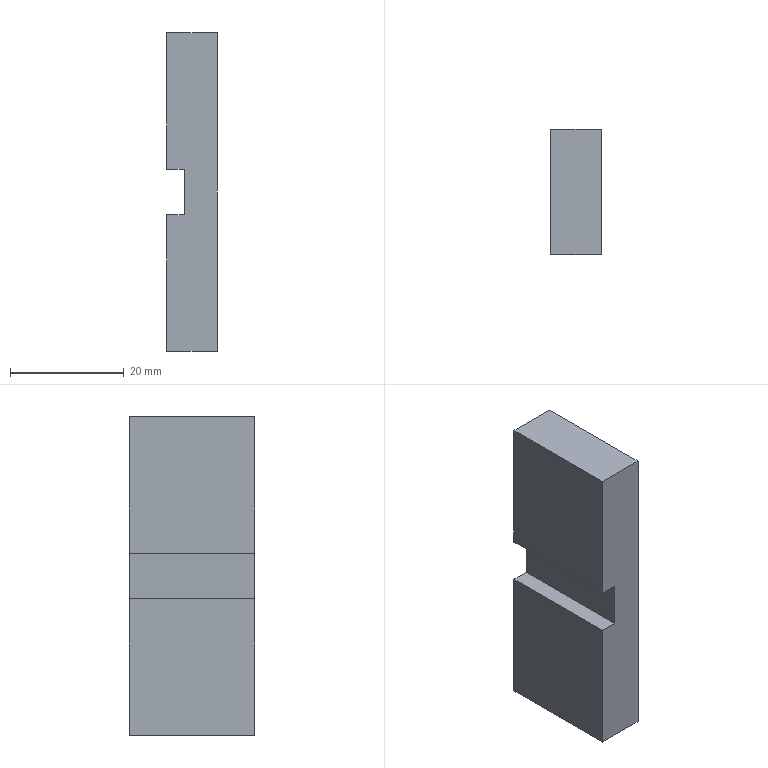Part | SolidWorks | features BaseBody 1 | 1 solid | 10 faces | box 8.8 x 22 x 56 mm | volume 10314 mm3 | plane 10
STEP:
#1=CARTESIAN_POINT('',(8.8,0.,-56.));
#2=VERTEX_POINT('',#1);
#3=CARTESIAN_POINT('',(8.8,0.,0.));
#4=VERTEX_POINT('',#3);
#5=CARTESIAN_POINT('',(8.8,0.,0.));
#6=DIRECTION('',(0.,0.,1.));
#7=VECTOR('',#6,1000.);
#8=LINE('',#5,#7);
#9=EDGE_CURVE('',#2,#4,#8,.T.);
#10=ORIENTED_EDGE('',*,*,#9,.F.);
#11=CARTESIAN_POINT('',(8.8,22.,-56.));
#12=VERTEX_POINT('',#11);
#13=CARTESIAN_POINT('',(8.8,0.,-56.));
#14=DIRECTION('',(0.,-1.,0.));
#15=VECTOR('',#14,1000.);
#16=LINE('',#13,#15);
#17=EDGE_CURVE('',#12,#2,#16,.T.);
#18=ORIENTED_EDGE('',*,*,#17,.F.);
#19=CARTESIAN_POINT('',(8.8,22.,0.));
#20=VERTEX_POINT('',#19);
#21=CARTESIAN_POINT('',(8.8,22.,0.));
#22=DIRECTION('',(0.,0.,-1.));
#23=VECTOR('',#22,1000.);
#24=LINE('',#21,#23);
#25=EDGE_CURVE('',#20,#12,#24,.T.);
#26=ORIENTED_EDGE('',*,*,#25,.F.);
#27=CARTESIAN_POINT('',(8.8,0.,0.));
#28=DIRECTION('',(0.,1.,0.));
#29=VECTOR('',#28,1000.);
#30=LINE('',#27,#29);
#31=EDGE_CURVE('',#4,#20,#30,.T.);
#32=ORIENTED_EDGE('',*,*,#31,.F.);
#33=EDGE_LOOP('',(#10,#18,#26,#32));
#34=FACE_OUTER_BOUND('',#33,.T.);
#35=CARTESIAN_POINT('',(8.8,0.,0.));
#36=DIRECTION('',(-1.,0.,0.));
#37=DIRECTION('',(0.,0.,1.));
#38=AXIS2_PLACEMENT_3D('',#35,#36,#37);
#39=PLANE('',#38);
#40=ADVANCED_FACE('',(#34),#39,.F.);
#41=CARTESIAN_POINT('',(0.,0.,0.));
#42=VERTEX_POINT('',#41);
#43=CARTESIAN_POINT('',(8.8,0.,0.));
#44=DIRECTION('',(-1.,0.,0.));
#45=VECTOR('',#44,1000.);
#46=LINE('',#43,#45);
#47=EDGE_CURVE('',#4,#42,#46,.T.);
#48=ORIENTED_EDGE('',*,*,#47,.F.);
#49=ORIENTED_EDGE('',*,*,#31,.T.);
#50=CARTESIAN_POINT('',(0.,22.,0.));
#51=VERTEX_POINT('',#50);
#52=CARTESIAN_POINT('',(8.8,22.,0.));
#53=DIRECTION('',(1.,0.,0.));
#54=VECTOR('',#53,1000.);
#55=LINE('',#52,#54);
#56=EDGE_CURVE('',#51,#20,#55,.T.);
#57=ORIENTED_EDGE('',*,*,#56,.F.);
#58=CARTESIAN_POINT('',(0.,0.,0.));
#59=DIRECTION('',(0.,1.,0.));
#60=VECTOR('',#59,1000.);
#61=LINE('',#58,#60);
#62=EDGE_CURVE('',#42,#51,#61,.T.);
#63=ORIENTED_EDGE('',*,*,#62,.F.);
#64=EDGE_LOOP('',(#48,#49,#57,#63));
#65=FACE_OUTER_BOUND('',#64,.T.);
#66=CARTESIAN_POINT('',(8.8,0.,0.));
#67=DIRECTION('',(0.,0.,-1.));
#68=DIRECTION('',(-1.,0.,0.));
#69=AXIS2_PLACEMENT_3D('',#66,#67,#68);
#70=PLANE('',#69);
#71=ADVANCED_FACE('',(#65),#70,.F.);
#72=CARTESIAN_POINT('',(0.,0.,-32.));
#73=VERTEX_POINT('',#72);
#74=CARTESIAN_POINT('',(3.,0.,-32.));
#75=VERTEX_POINT('',#74);
#76=CARTESIAN_POINT('',(8.8,0.,-32.));
#77=DIRECTION('',(1.,0.,0.));
#78=VECTOR('',#77,1000.);
#79=LINE('',#76,#78);
#80=EDGE_CURVE('',#73,#75,#79,.T.);
#81=ORIENTED_EDGE('',*,*,#80,.F.);
#82=CARTESIAN_POINT('',(0.,0.,-56.));
#83=VERTEX_POINT('',#82);
#84=CARTESIAN_POINT('',(0.,0.,0.));
#85=DIRECTION('',(0.,0.,1.));
#86=VECTOR('',#85,1000.);
#87=LINE('',#84,#86);
#88=EDGE_CURVE('',#83,#73,#87,.T.);
#89=ORIENTED_EDGE('',*,*,#88,.F.);
#90=CARTESIAN_POINT('',(8.8,0.,-56.));
#91=DIRECTION('',(-1.,0.,0.));
#92=VECTOR('',#91,1000.);
#93=LINE('',#90,#92);
#94=EDGE_CURVE('',#2,#83,#93,.T.);
#95=ORIENTED_EDGE('',*,*,#94,.F.);
#96=ORIENTED_EDGE('',*,*,#9,.T.);
#97=ORIENTED_EDGE('',*,*,#47,.T.);
#98=CARTESIAN_POINT('',(0.,0.,-24.));
#99=VERTEX_POINT('',#98);
#100=CARTESIAN_POINT('',(0.,0.,0.));
#101=DIRECTION('',(0.,0.,1.));
#102=VECTOR('',#101,1000.);
#103=LINE('',#100,#102);
#104=EDGE_CURVE('',#99,#42,#103,.T.);
#105=ORIENTED_EDGE('',*,*,#104,.F.);
#106=CARTESIAN_POINT('',(3.,0.,-24.));
#107=VERTEX_POINT('',#106);
#108=CARTESIAN_POINT('',(8.8,0.,-24.));
#109=DIRECTION('',(-1.,0.,0.));
#110=VECTOR('',#109,1000.);
#111=LINE('',#108,#110);
#112=EDGE_CURVE('',#107,#99,#111,.T.);
#113=ORIENTED_EDGE('',*,*,#112,.F.);
#114=CARTESIAN_POINT('',(3.,0.,0.));
#115=DIRECTION('',(0.,0.,1.));
#116=VECTOR('',#115,1000.);
#117=LINE('',#114,#116);
#118=EDGE_CURVE('',#75,#107,#117,.T.);
#119=ORIENTED_EDGE('',*,*,#118,.F.);
#120=EDGE_LOOP('',(#81,#89,#95,#96,#97,#105,#113,#119));
#121=FACE_OUTER_BOUND('',#120,.T.);
#122=CARTESIAN_POINT('',(8.8,0.,0.));
#123=DIRECTION('',(0.,1.,0.));
#124=DIRECTION('',(0.,0.,1.));
#125=AXIS2_PLACEMENT_3D('',#122,#123,#124);
#126=PLANE('',#125);
#127=ADVANCED_FACE('',(#121),#126,.F.);
#128=CARTESIAN_POINT('',(0.,22.,-56.));
#129=VERTEX_POINT('',#128);
#130=CARTESIAN_POINT('',(8.8,22.,-56.));
#131=DIRECTION('',(-1.,0.,0.));
#132=VECTOR('',#131,1000.);
#133=LINE('',#130,#132);
#134=EDGE_CURVE('',#12,#129,#133,.T.);
#135=ORIENTED_EDGE('',*,*,#134,.F.);
#136=ORIENTED_EDGE('',*,*,#17,.T.);
#137=ORIENTED_EDGE('',*,*,#94,.T.);
#138=CARTESIAN_POINT('',(0.,0.,-56.));
#139=DIRECTION('',(0.,-1.,0.));
#140=VECTOR('',#139,1000.);
#141=LINE('',#138,#140);
#142=EDGE_CURVE('',#129,#83,#141,.T.);
#143=ORIENTED_EDGE('',*,*,#142,.F.);
#144=EDGE_LOOP('',(#135,#136,#137,#143));
#145=FACE_OUTER_BOUND('',#144,.T.);
#146=CARTESIAN_POINT('',(8.8,0.,-56.));
#147=DIRECTION('',(0.,0.,1.));
#148=DIRECTION('',(1.,0.,0.));
#149=AXIS2_PLACEMENT_3D('',#146,#147,#148);
#150=PLANE('',#149);
#151=ADVANCED_FACE('',(#145),#150,.F.);
#152=CARTESIAN_POINT('',(3.,22.,-32.));
#153=VERTEX_POINT('',#152);
#154=CARTESIAN_POINT('',(0.,22.,-32.));
#155=VERTEX_POINT('',#154);
#156=CARTESIAN_POINT('',(8.8,22.,-32.));
#157=DIRECTION('',(-1.,0.,0.));
#158=VECTOR('',#157,1000.);
#159=LINE('',#156,#158);
#160=EDGE_CURVE('',#153,#155,#159,.T.);
#161=ORIENTED_EDGE('',*,*,#160,.F.);
#162=CARTESIAN_POINT('',(3.,22.,-24.));
#163=VERTEX_POINT('',#162);
#164=CARTESIAN_POINT('',(3.,22.,0.));
#165=DIRECTION('',(0.,0.,-1.));
#166=VECTOR('',#165,1000.);
#167=LINE('',#164,#166);
#168=EDGE_CURVE('',#163,#153,#167,.T.);
#169=ORIENTED_EDGE('',*,*,#168,.F.);
#170=CARTESIAN_POINT('',(0.,22.,-24.));
#171=VERTEX_POINT('',#170);
#172=CARTESIAN_POINT('',(8.8,22.,-24.));
#173=DIRECTION('',(1.,0.,0.));
#174=VECTOR('',#173,1000.);
#175=LINE('',#172,#174);
#176=EDGE_CURVE('',#171,#163,#175,.T.);
#177=ORIENTED_EDGE('',*,*,#176,.F.);
#178=CARTESIAN_POINT('',(0.,22.,0.));
#179=DIRECTION('',(0.,0.,-1.));
#180=VECTOR('',#179,1000.);
#181=LINE('',#178,#180);
#182=EDGE_CURVE('',#51,#171,#181,.T.);
#183=ORIENTED_EDGE('',*,*,#182,.F.);
#184=ORIENTED_EDGE('',*,*,#56,.T.);
#185=ORIENTED_EDGE('',*,*,#25,.T.);
#186=ORIENTED_EDGE('',*,*,#134,.T.);
#187=CARTESIAN_POINT('',(0.,22.,0.));
#188=DIRECTION('',(0.,0.,-1.));
#189=VECTOR('',#188,1000.);
#190=LINE('',#187,#189);
#191=EDGE_CURVE('',#155,#129,#190,.T.);
#192=ORIENTED_EDGE('',*,*,#191,.F.);
#193=EDGE_LOOP('',(#161,#169,#177,#183,#184,#185,#186,#192));
#194=FACE_OUTER_BOUND('',#193,.T.);
#195=CARTESIAN_POINT('',(8.8,22.,0.));
#196=DIRECTION('',(0.,-1.,0.));
#197=DIRECTION('',(0.,0.,-1.));
#198=AXIS2_PLACEMENT_3D('',#195,#196,#197);
#199=PLANE('',#198);
#200=ADVANCED_FACE('',(#194),#199,.F.);
#201=ORIENTED_EDGE('',*,*,#62,.T.);
#202=ORIENTED_EDGE('',*,*,#182,.T.);
#203=CARTESIAN_POINT('',(0.,0.,-24.));
#204=DIRECTION('',(0.,-1.,0.));
#205=VECTOR('',#204,1000.);
#206=LINE('',#203,#205);
#207=EDGE_CURVE('',#171,#99,#206,.T.);
#208=ORIENTED_EDGE('',*,*,#207,.T.);
#209=ORIENTED_EDGE('',*,*,#104,.T.);
#210=EDGE_LOOP('',(#201,#202,#208,#209));
#211=FACE_OUTER_BOUND('',#210,.T.);
#212=CARTESIAN_POINT('',(0.,0.,0.));
#213=DIRECTION('',(-1.,0.,0.));
#214=DIRECTION('',(0.,0.,1.));
#215=AXIS2_PLACEMENT_3D('',#212,#213,#214);
#216=PLANE('',#215);
#217=ADVANCED_FACE('',(#211),#216,.T.);
#218=ORIENTED_EDGE('',*,*,#168,.T.);
#219=CARTESIAN_POINT('',(3.,0.,-32.));
#220=DIRECTION('',(0.,-1.,0.));
#221=VECTOR('',#220,1000.);
#222=LINE('',#219,#221);
#223=EDGE_CURVE('',#153,#75,#222,.T.);
#224=ORIENTED_EDGE('',*,*,#223,.T.);
#225=ORIENTED_EDGE('',*,*,#118,.T.);
#226=CARTESIAN_POINT('',(3.,0.,-24.));
#227=DIRECTION('',(0.,1.,0.));
#228=VECTOR('',#227,1000.);
#229=LINE('',#226,#228);
#230=EDGE_CURVE('',#107,#163,#229,.T.);
#231=ORIENTED_EDGE('',*,*,#230,.T.);
#232=EDGE_LOOP('',(#218,#224,#225,#231));
#233=FACE_OUTER_BOUND('',#232,.T.);
#234=CARTESIAN_POINT('',(3.,0.,0.));
#235=DIRECTION('',(-1.,0.,0.));
#236=DIRECTION('',(0.,0.,1.));
#237=AXIS2_PLACEMENT_3D('',#234,#235,#236);
#238=PLANE('',#237);
#239=ADVANCED_FACE('',(#233),#238,.T.);
#240=ORIENTED_EDGE('',*,*,#160,.T.);
#241=CARTESIAN_POINT('',(0.,28.365,-32.));
#242=DIRECTION('',(0.,1.,0.));
#243=VECTOR('',#242,1000.);
#244=LINE('',#241,#243);
#245=EDGE_CURVE('',#73,#155,#244,.T.);
#246=ORIENTED_EDGE('',*,*,#245,.F.);
#247=ORIENTED_EDGE('',*,*,#80,.T.);
#248=ORIENTED_EDGE('',*,*,#223,.F.);
#249=EDGE_LOOP('',(#240,#246,#247,#248));
#250=FACE_OUTER_BOUND('',#249,.T.);
#251=CARTESIAN_POINT('',(3.,28.365,-32.));
#252=DIRECTION('',(0.,0.,-1.));
#253=DIRECTION('',(0.,1.,0.));
#254=AXIS2_PLACEMENT_3D('',#251,#252,#253);
#255=PLANE('',#254);
#256=ADVANCED_FACE('',(#250),#255,.F.);
#257=ORIENTED_EDGE('',*,*,#142,.T.);
#258=ORIENTED_EDGE('',*,*,#88,.T.);
#259=ORIENTED_EDGE('',*,*,#245,.T.);
#260=ORIENTED_EDGE('',*,*,#191,.T.);
#261=EDGE_LOOP('',(#257,#258,#259,#260));
#262=FACE_OUTER_BOUND('',#261,.T.);
#263=CARTESIAN_POINT('',(0.,0.,0.));
#264=DIRECTION('',(-1.,0.,0.));
#265=DIRECTION('',(0.,0.,1.));
#266=AXIS2_PLACEMENT_3D('',#263,#264,#265);
#267=PLANE('',#266);
#268=ADVANCED_FACE('',(#262),#267,.T.);
#269=ORIENTED_EDGE('',*,*,#176,.T.);
#270=ORIENTED_EDGE('',*,*,#230,.F.);
#271=ORIENTED_EDGE('',*,*,#112,.T.);
#272=ORIENTED_EDGE('',*,*,#207,.F.);
#273=EDGE_LOOP('',(#269,#270,#271,#272));
#274=FACE_OUTER_BOUND('',#273,.T.);
#275=CARTESIAN_POINT('',(3.,28.365,-24.));
#276=DIRECTION('',(0.,0.,1.));
#277=DIRECTION('',(0.,-1.,0.));
#278=AXIS2_PLACEMENT_3D('',#275,#276,#277);
#279=PLANE('',#278);
#280=ADVANCED_FACE('',(#274),#279,.F.);
#281=CLOSED_SHELL('',(#40,#71,#127,#151,#200,#217,#239,#256,#268,#280));
#282=MANIFOLD_SOLID_BREP('',#281);
#283=CARTESIAN_POINT('',(0.,0.,0.));
#284=DIRECTION('',(0.,0.,1.));
#285=DIRECTION('',(1.,0.,0.));
#286=AXIS2_PLACEMENT_3D('',#283,#284,#285);
#287=(LENGTH_UNIT()NAMED_UNIT(*)SI_UNIT(.MILLI.,.METRE.));
#288=UNCERTAINTY_MEASURE_WITH_UNIT(LENGTH_MEASURE(0.00001),#287,'','');
#289=(NAMED_UNIT(*)PLANE_ANGLE_UNIT()SI_UNIT($,.RADIAN.));
#290=(NAMED_UNIT(*)SI_UNIT($,.STERADIAN.)SOLID_ANGLE_UNIT());
#291=(GEOMETRIC_REPRESENTATION_CONTEXT(3)GLOBAL_UNCERTAINTY_ASSIGNED_CONTEXT((#288))GLOBAL_UNIT_ASSIGNED_CONTEXT((#287,#289,#290))REPRESENTATION_CONTEXT('',''));
#292=ADVANCED_BREP_SHAPE_REPRESENTATION('',(#282,#286),#291);